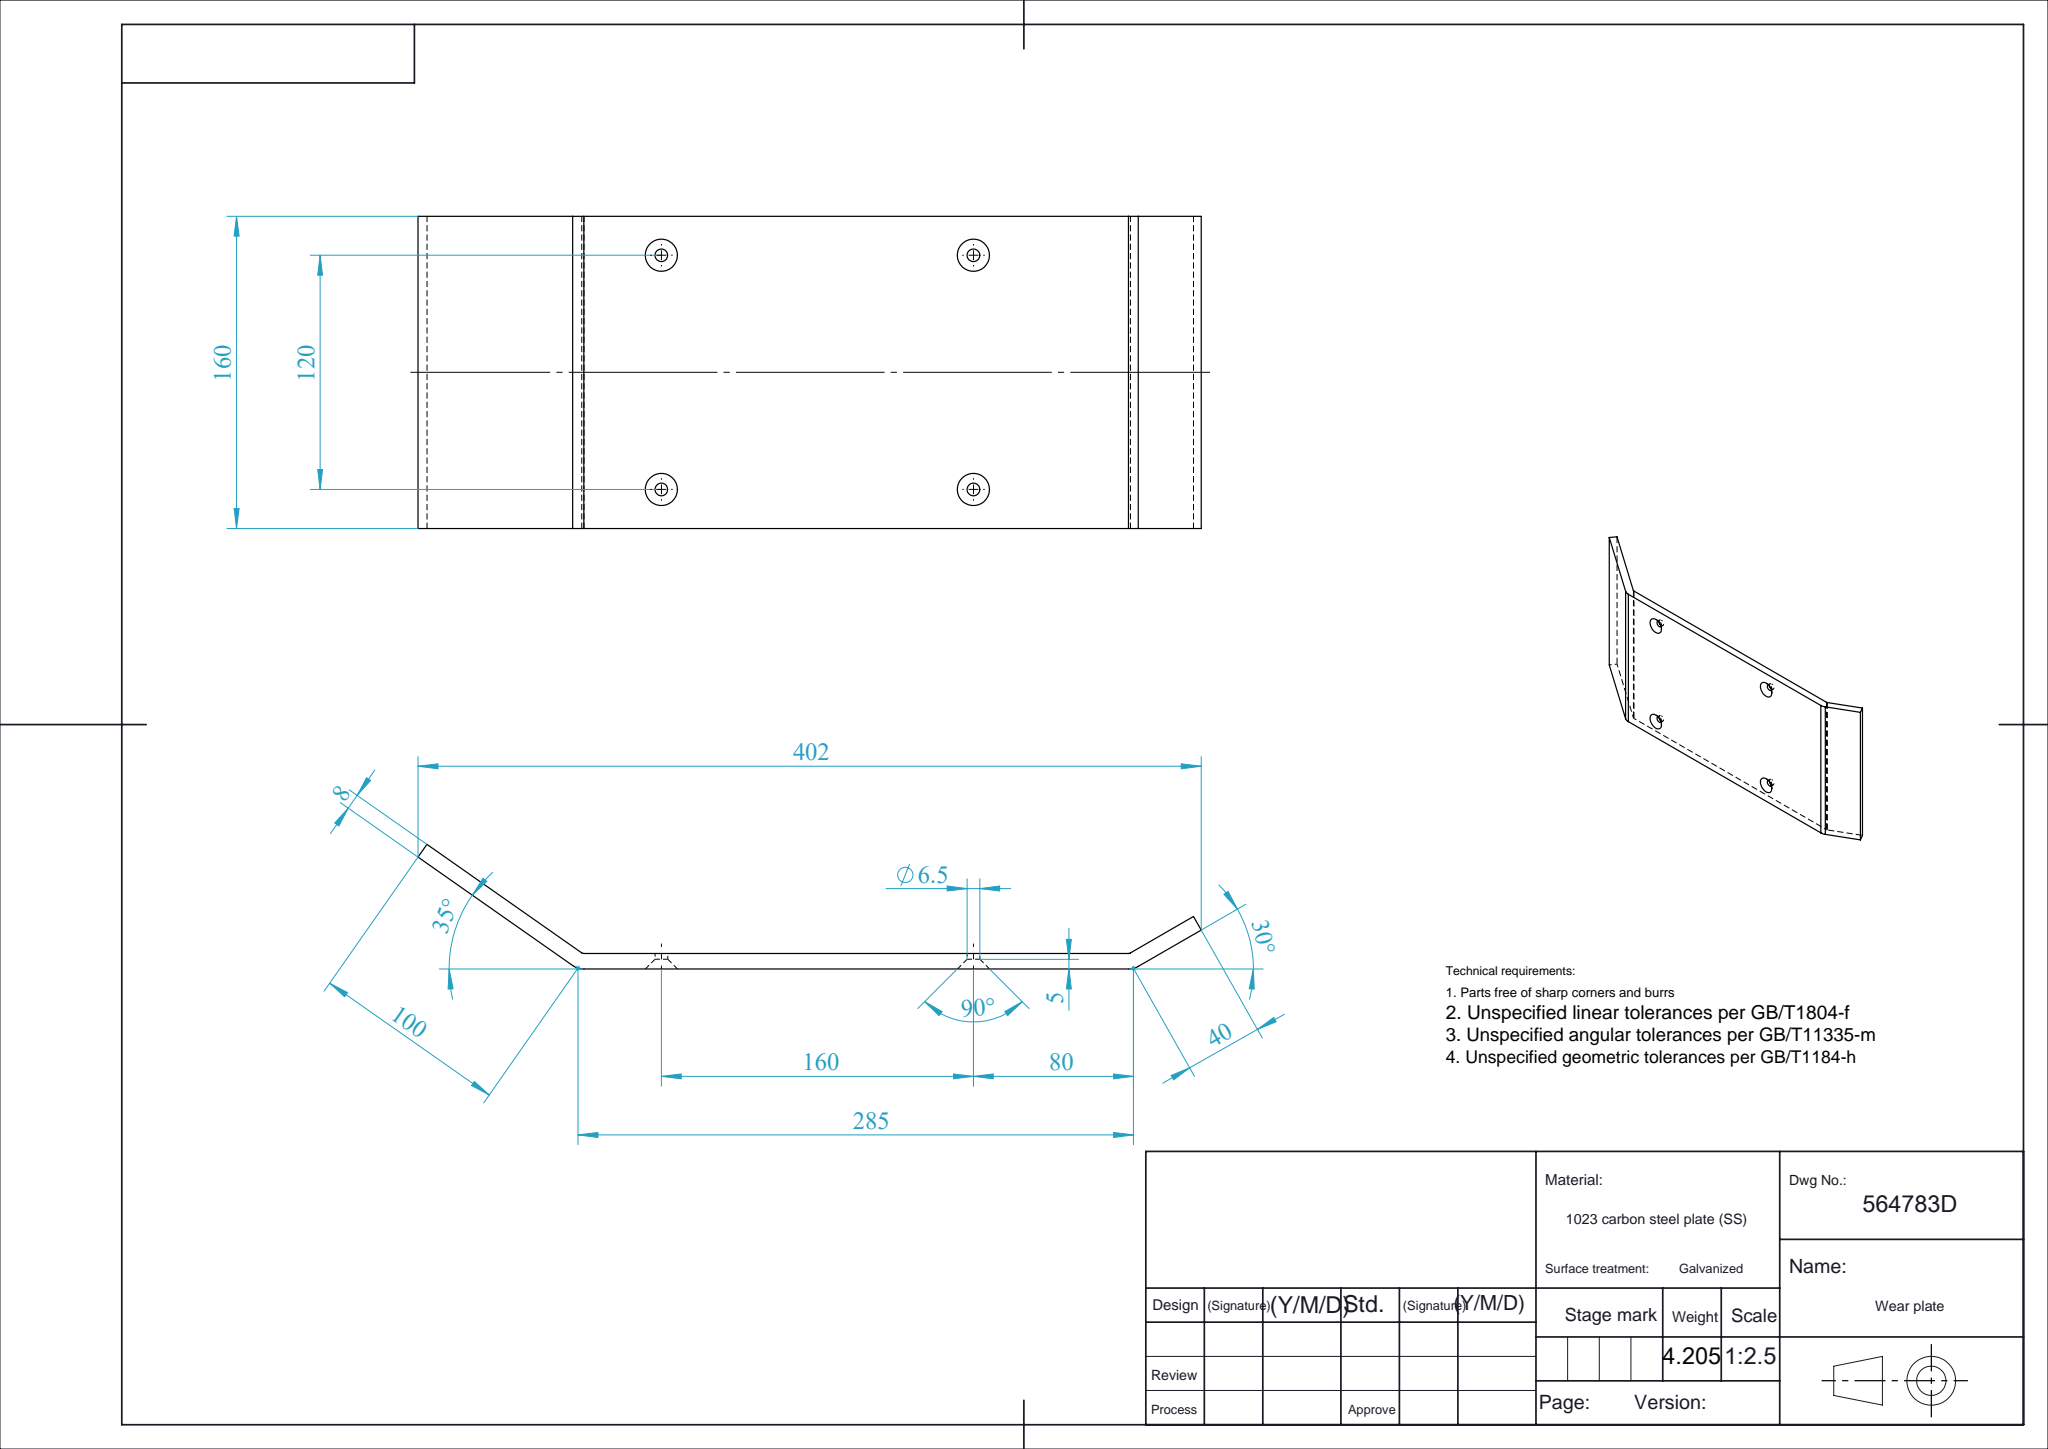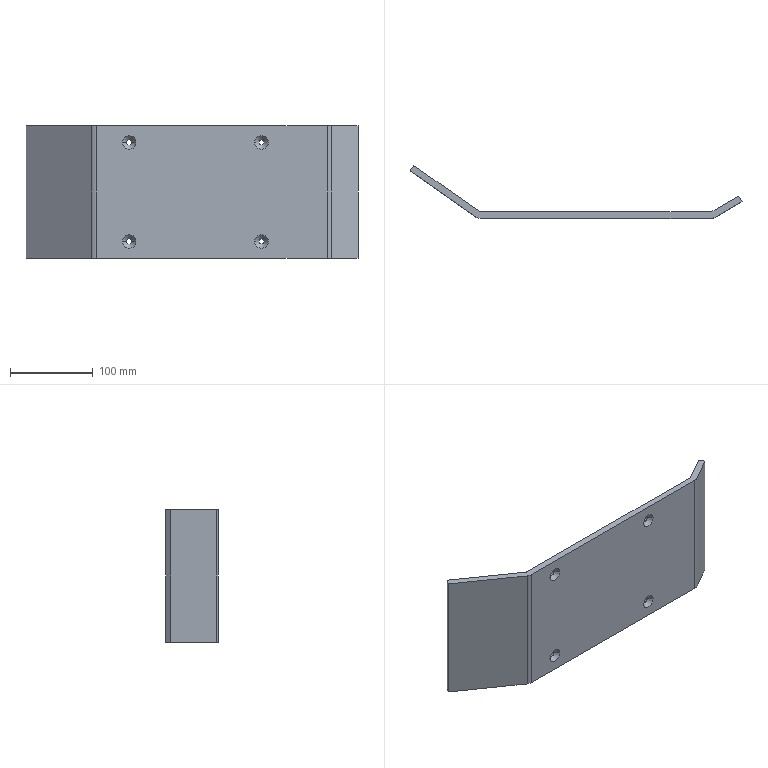Part | SolidWorks | features Fillet 2, ICE 2, Extrusion 1 | 1 solid | 30 faces | box 401.556 x 63.911 x 160 mm | volume 535175 mm3 | cylinder 12 | plane 10 | cone 8 | commonest cylinder face diameters 6.5 x8 4 x2 20 x2
STEP:
#1=CARTESIAN_POINT('',(121.522,-52.358,20.));
#2=VERTEX_POINT('',#1);
#3=CARTESIAN_POINT('',(124.772,-52.358,16.75));
#4=VERTEX_POINT('',#3);
#5=CARTESIAN_POINT('',(124.772,-52.358,20.));
#6=DIRECTION('',(0.,-1.,0.));
#7=DIRECTION('',(1.,0.,0.));
#8=AXIS2_PLACEMENT_3D('',#5,#6,#7);
#9=CIRCLE('',#8,3.25);
#10=EDGE_CURVE('',#2,#4,#9,.T.);
#11=ORIENTED_EDGE('',*,*,#10,.F.);
#12=CARTESIAN_POINT('',(116.522,-57.358,20.));
#13=VERTEX_POINT('',#12);
#14=CARTESIAN_POINT('',(116.522,-57.358,20.));
#15=DIRECTION('',(-0.7071,-0.7071,0.));
#16=VECTOR('',#15,1000.);
#17=LINE('',#14,#16);
#18=EDGE_CURVE('',#2,#13,#17,.T.);
#19=ORIENTED_EDGE('',*,*,#18,.T.);
#20=CARTESIAN_POINT('',(133.022,-57.358,20.));
#21=VERTEX_POINT('',#20);
#22=CARTESIAN_POINT('',(124.772,-57.358,20.));
#23=DIRECTION('',(0.,-1.,0.));
#24=DIRECTION('',(1.,0.,0.));
#25=AXIS2_PLACEMENT_3D('',#22,#23,#24);
#26=CIRCLE('',#25,8.25);
#27=EDGE_CURVE('',#13,#21,#26,.T.);
#28=ORIENTED_EDGE('',*,*,#27,.T.);
#29=CARTESIAN_POINT('',(128.022,-52.358,20.));
#30=VERTEX_POINT('',#29);
#31=CARTESIAN_POINT('',(133.022,-57.358,20.));
#32=DIRECTION('',(0.7071,-0.7071,0.));
#33=VECTOR('',#32,1000.);
#34=LINE('',#31,#33);
#35=EDGE_CURVE('',#30,#21,#34,.T.);
#36=ORIENTED_EDGE('',*,*,#35,.F.);
#37=CARTESIAN_POINT('',(124.772,-52.358,20.));
#38=DIRECTION('',(0.,-1.,0.));
#39=DIRECTION('',(1.,0.,0.));
#40=AXIS2_PLACEMENT_3D('',#37,#38,#39);
#41=CIRCLE('',#40,3.25);
#42=EDGE_CURVE('',#4,#30,#41,.T.);
#43=ORIENTED_EDGE('',*,*,#42,.F.);
#44=EDGE_LOOP('',(#11,#19,#28,#36,#43));
#45=FACE_OUTER_BOUND('',#44,.T.);
#46=CARTESIAN_POINT('',(124.772,-57.358,20.));
#47=DIRECTION('',(0.,-1.,0.));
#48=DIRECTION('',(1.,0.,0.));
#49=AXIS2_PLACEMENT_3D('',#46,#47,#48);
#50=CONICAL_SURFACE('',#49,8.25,0.7854);
#51=ADVANCED_FACE('',(#45),#50,.F.);
#52=CARTESIAN_POINT('',(281.522,-52.358,140.));
#53=VERTEX_POINT('',#52);
#54=CARTESIAN_POINT('',(284.772,-52.358,136.75));
#55=VERTEX_POINT('',#54);
#56=CARTESIAN_POINT('',(284.772,-52.358,140.));
#57=DIRECTION('',(0.,-1.,0.));
#58=DIRECTION('',(1.,0.,0.));
#59=AXIS2_PLACEMENT_3D('',#56,#57,#58);
#60=CIRCLE('',#59,3.25);
#61=EDGE_CURVE('',#53,#55,#60,.T.);
#62=ORIENTED_EDGE('',*,*,#61,.F.);
#63=CARTESIAN_POINT('',(276.522,-57.358,140.));
#64=VERTEX_POINT('',#63);
#65=CARTESIAN_POINT('',(276.522,-57.358,140.));
#66=DIRECTION('',(-0.7071,-0.7071,0.));
#67=VECTOR('',#66,1000.);
#68=LINE('',#65,#67);
#69=EDGE_CURVE('',#53,#64,#68,.T.);
#70=ORIENTED_EDGE('',*,*,#69,.T.);
#71=CARTESIAN_POINT('',(293.022,-57.358,140.));
#72=VERTEX_POINT('',#71);
#73=CARTESIAN_POINT('',(284.772,-57.358,140.));
#74=DIRECTION('',(0.,-1.,0.));
#75=DIRECTION('',(1.,0.,0.));
#76=AXIS2_PLACEMENT_3D('',#73,#74,#75);
#77=CIRCLE('',#76,8.25);
#78=EDGE_CURVE('',#64,#72,#77,.T.);
#79=ORIENTED_EDGE('',*,*,#78,.T.);
#80=CARTESIAN_POINT('',(288.022,-52.358,140.));
#81=VERTEX_POINT('',#80);
#82=CARTESIAN_POINT('',(293.022,-57.358,140.));
#83=DIRECTION('',(0.7071,-0.7071,0.));
#84=VECTOR('',#83,1000.);
#85=LINE('',#82,#84);
#86=EDGE_CURVE('',#81,#72,#85,.T.);
#87=ORIENTED_EDGE('',*,*,#86,.F.);
#88=CARTESIAN_POINT('',(284.772,-52.358,140.));
#89=DIRECTION('',(0.,-1.,0.));
#90=DIRECTION('',(1.,0.,0.));
#91=AXIS2_PLACEMENT_3D('',#88,#89,#90);
#92=CIRCLE('',#91,3.25);
#93=EDGE_CURVE('',#55,#81,#92,.T.);
#94=ORIENTED_EDGE('',*,*,#93,.F.);
#95=EDGE_LOOP('',(#62,#70,#79,#87,#94));
#96=FACE_OUTER_BOUND('',#95,.T.);
#97=CARTESIAN_POINT('',(284.772,-57.358,140.));
#98=DIRECTION('',(0.,-1.,0.));
#99=DIRECTION('',(1.,0.,0.));
#100=AXIS2_PLACEMENT_3D('',#97,#98,#99);
#101=CONICAL_SURFACE('',#100,8.25,0.7854);
#102=ADVANCED_FACE('',(#96),#101,.F.);
#103=CARTESIAN_POINT('',(121.522,-52.358,140.));
#104=VERTEX_POINT('',#103);
#105=CARTESIAN_POINT('',(124.772,-52.358,136.75));
#106=VERTEX_POINT('',#105);
#107=CARTESIAN_POINT('',(124.772,-52.358,140.));
#108=DIRECTION('',(0.,-1.,0.));
#109=DIRECTION('',(1.,0.,0.));
#110=AXIS2_PLACEMENT_3D('',#107,#108,#109);
#111=CIRCLE('',#110,3.25);
#112=EDGE_CURVE('',#104,#106,#111,.T.);
#113=ORIENTED_EDGE('',*,*,#112,.F.);
#114=CARTESIAN_POINT('',(116.522,-57.358,140.));
#115=VERTEX_POINT('',#114);
#116=CARTESIAN_POINT('',(116.522,-57.358,140.));
#117=DIRECTION('',(-0.7071,-0.7071,0.));
#118=VECTOR('',#117,1000.);
#119=LINE('',#116,#118);
#120=EDGE_CURVE('',#104,#115,#119,.T.);
#121=ORIENTED_EDGE('',*,*,#120,.T.);
#122=CARTESIAN_POINT('',(133.022,-57.358,140.));
#123=VERTEX_POINT('',#122);
#124=CARTESIAN_POINT('',(124.772,-57.358,140.));
#125=DIRECTION('',(0.,-1.,0.));
#126=DIRECTION('',(1.,0.,0.));
#127=AXIS2_PLACEMENT_3D('',#124,#125,#126);
#128=CIRCLE('',#127,8.25);
#129=EDGE_CURVE('',#115,#123,#128,.T.);
#130=ORIENTED_EDGE('',*,*,#129,.T.);
#131=CARTESIAN_POINT('',(128.022,-52.358,140.));
#132=VERTEX_POINT('',#131);
#133=CARTESIAN_POINT('',(133.022,-57.358,140.));
#134=DIRECTION('',(0.7071,-0.7071,0.));
#135=VECTOR('',#134,1000.);
#136=LINE('',#133,#135);
#137=EDGE_CURVE('',#132,#123,#136,.T.);
#138=ORIENTED_EDGE('',*,*,#137,.F.);
#139=CARTESIAN_POINT('',(124.772,-52.358,140.));
#140=DIRECTION('',(0.,-1.,0.));
#141=DIRECTION('',(1.,0.,0.));
#142=AXIS2_PLACEMENT_3D('',#139,#140,#141);
#143=CIRCLE('',#142,3.25);
#144=EDGE_CURVE('',#106,#132,#143,.T.);
#145=ORIENTED_EDGE('',*,*,#144,.F.);
#146=EDGE_LOOP('',(#113,#121,#130,#138,#145));
#147=FACE_OUTER_BOUND('',#146,.T.);
#148=CARTESIAN_POINT('',(124.772,-57.358,140.));
#149=DIRECTION('',(0.,-1.,0.));
#150=DIRECTION('',(1.,0.,0.));
#151=AXIS2_PLACEMENT_3D('',#148,#149,#150);
#152=CONICAL_SURFACE('',#151,8.25,0.7854);
#153=ADVANCED_FACE('',(#147),#152,.F.);
#154=CARTESIAN_POINT('',(281.522,-52.358,20.));
#155=VERTEX_POINT('',#154);
#156=CARTESIAN_POINT('',(284.772,-52.358,16.75));
#157=VERTEX_POINT('',#156);
#158=CARTESIAN_POINT('',(284.772,-52.358,20.));
#159=DIRECTION('',(0.,-1.,0.));
#160=DIRECTION('',(1.,0.,0.));
#161=AXIS2_PLACEMENT_3D('',#158,#159,#160);
#162=CIRCLE('',#161,3.25);
#163=EDGE_CURVE('',#155,#157,#162,.T.);
#164=ORIENTED_EDGE('',*,*,#163,.F.);
#165=CARTESIAN_POINT('',(276.522,-57.358,20.));
#166=VERTEX_POINT('',#165);
#167=CARTESIAN_POINT('',(276.522,-57.358,20.));
#168=DIRECTION('',(-0.7071,-0.7071,0.));
#169=VECTOR('',#168,1000.);
#170=LINE('',#167,#169);
#171=EDGE_CURVE('',#155,#166,#170,.T.);
#172=ORIENTED_EDGE('',*,*,#171,.T.);
#173=CARTESIAN_POINT('',(293.022,-57.358,20.));
#174=VERTEX_POINT('',#173);
#175=CARTESIAN_POINT('',(284.772,-57.358,20.));
#176=DIRECTION('',(0.,-1.,0.));
#177=DIRECTION('',(1.,0.,0.));
#178=AXIS2_PLACEMENT_3D('',#175,#176,#177);
#179=CIRCLE('',#178,8.25);
#180=EDGE_CURVE('',#166,#174,#179,.T.);
#181=ORIENTED_EDGE('',*,*,#180,.T.);
#182=CARTESIAN_POINT('',(288.022,-52.358,20.));
#183=VERTEX_POINT('',#182);
#184=CARTESIAN_POINT('',(293.022,-57.358,20.));
#185=DIRECTION('',(0.7071,-0.7071,0.));
#186=VECTOR('',#185,1000.);
#187=LINE('',#184,#186);
#188=EDGE_CURVE('',#183,#174,#187,.T.);
#189=ORIENTED_EDGE('',*,*,#188,.F.);
#190=CARTESIAN_POINT('',(284.772,-52.358,20.));
#191=DIRECTION('',(0.,-1.,0.));
#192=DIRECTION('',(1.,0.,0.));
#193=AXIS2_PLACEMENT_3D('',#190,#191,#192);
#194=CIRCLE('',#193,3.25);
#195=EDGE_CURVE('',#157,#183,#194,.T.);
#196=ORIENTED_EDGE('',*,*,#195,.F.);
#197=EDGE_LOOP('',(#164,#172,#181,#189,#196));
#198=FACE_OUTER_BOUND('',#197,.T.);
#199=CARTESIAN_POINT('',(284.772,-57.358,20.));
#200=DIRECTION('',(0.,-1.,0.));
#201=DIRECTION('',(1.,0.,0.));
#202=AXIS2_PLACEMENT_3D('',#199,#200,#201);
#203=CONICAL_SURFACE('',#202,8.25,0.7854);
#204=ADVANCED_FACE('',(#198),#203,.F.);
#205=CARTESIAN_POINT('',(284.772,-52.358,23.25));
#206=VERTEX_POINT('',#205);
#207=CARTESIAN_POINT('',(284.772,-52.358,20.));
#208=DIRECTION('',(0.,-1.,0.));
#209=DIRECTION('',(1.,0.,0.));
#210=AXIS2_PLACEMENT_3D('',#207,#208,#209);
#211=CIRCLE('',#210,3.25);
#212=EDGE_CURVE('',#206,#155,#211,.T.);
#213=ORIENTED_EDGE('',*,*,#212,.T.);
#214=ORIENTED_EDGE('',*,*,#163,.T.);
#215=CARTESIAN_POINT('',(284.772,-49.358,16.75));
#216=VERTEX_POINT('',#215);
#217=CARTESIAN_POINT('',(284.772,-57.358,16.75));
#218=DIRECTION('',(0.,1.,0.));
#219=VECTOR('',#218,1000.);
#220=LINE('',#217,#219);
#221=EDGE_CURVE('',#157,#216,#220,.T.);
#222=ORIENTED_EDGE('',*,*,#221,.T.);
#223=CARTESIAN_POINT('',(284.772,-49.358,23.25));
#224=VERTEX_POINT('',#223);
#225=CARTESIAN_POINT('',(284.772,-49.358,20.));
#226=DIRECTION('',(0.,1.,0.));
#227=DIRECTION('',(0.,0.,1.));
#228=AXIS2_PLACEMENT_3D('',#225,#226,#227);
#229=CIRCLE('',#228,3.25);
#230=EDGE_CURVE('',#216,#224,#229,.T.);
#231=ORIENTED_EDGE('',*,*,#230,.T.);
#232=CARTESIAN_POINT('',(284.772,-57.358,23.25));
#233=DIRECTION('',(0.,1.,0.));
#234=VECTOR('',#233,1000.);
#235=LINE('',#232,#234);
#236=EDGE_CURVE('',#206,#224,#235,.T.);
#237=ORIENTED_EDGE('',*,*,#236,.F.);
#238=EDGE_LOOP('',(#213,#214,#222,#231,#237));
#239=FACE_OUTER_BOUND('',#238,.T.);
#240=CARTESIAN_POINT('',(284.772,-57.358,20.));
#241=DIRECTION('',(0.,1.,0.));
#242=DIRECTION('',(0.,0.,1.));
#243=AXIS2_PLACEMENT_3D('',#240,#241,#242);
#244=CYLINDRICAL_SURFACE('',#243,3.25);
#245=ADVANCED_FACE('',(#239),#244,.F.);
#246=CARTESIAN_POINT('',(124.772,-52.358,143.25));
#247=VERTEX_POINT('',#246);
#248=CARTESIAN_POINT('',(124.772,-52.358,140.));
#249=DIRECTION('',(0.,-1.,0.));
#250=DIRECTION('',(1.,0.,0.));
#251=AXIS2_PLACEMENT_3D('',#248,#249,#250);
#252=CIRCLE('',#251,3.25);
#253=EDGE_CURVE('',#247,#104,#252,.T.);
#254=ORIENTED_EDGE('',*,*,#253,.T.);
#255=ORIENTED_EDGE('',*,*,#112,.T.);
#256=CARTESIAN_POINT('',(124.772,-49.358,136.75));
#257=VERTEX_POINT('',#256);
#258=CARTESIAN_POINT('',(124.772,-57.358,136.75));
#259=DIRECTION('',(0.,1.,0.));
#260=VECTOR('',#259,1000.);
#261=LINE('',#258,#260);
#262=EDGE_CURVE('',#106,#257,#261,.T.);
#263=ORIENTED_EDGE('',*,*,#262,.T.);
#264=CARTESIAN_POINT('',(124.772,-49.358,143.25));
#265=VERTEX_POINT('',#264);
#266=CARTESIAN_POINT('',(124.772,-49.358,140.));
#267=DIRECTION('',(0.,1.,0.));
#268=DIRECTION('',(0.,0.,1.));
#269=AXIS2_PLACEMENT_3D('',#266,#267,#268);
#270=CIRCLE('',#269,3.25);
#271=EDGE_CURVE('',#257,#265,#270,.T.);
#272=ORIENTED_EDGE('',*,*,#271,.T.);
#273=CARTESIAN_POINT('',(124.772,-57.358,143.25));
#274=DIRECTION('',(0.,1.,0.));
#275=VECTOR('',#274,1000.);
#276=LINE('',#273,#275);
#277=EDGE_CURVE('',#247,#265,#276,.T.);
#278=ORIENTED_EDGE('',*,*,#277,.F.);
#279=EDGE_LOOP('',(#254,#255,#263,#272,#278));
#280=FACE_OUTER_BOUND('',#279,.T.);
#281=CARTESIAN_POINT('',(124.772,-57.358,140.));
#282=DIRECTION('',(0.,1.,0.));
#283=DIRECTION('',(0.,0.,1.));
#284=AXIS2_PLACEMENT_3D('',#281,#282,#283);
#285=CYLINDRICAL_SURFACE('',#284,3.25);
#286=ADVANCED_FACE('',(#280),#285,.F.);
#287=CARTESIAN_POINT('',(284.772,-52.358,143.25));
#288=VERTEX_POINT('',#287);
#289=CARTESIAN_POINT('',(284.772,-52.358,140.));
#290=DIRECTION('',(0.,-1.,0.));
#291=DIRECTION('',(1.,0.,0.));
#292=AXIS2_PLACEMENT_3D('',#289,#290,#291);
#293=CIRCLE('',#292,3.25);
#294=EDGE_CURVE('',#288,#53,#293,.T.);
#295=ORIENTED_EDGE('',*,*,#294,.T.);
#296=ORIENTED_EDGE('',*,*,#61,.T.);
#297=CARTESIAN_POINT('',(284.772,-49.358,136.75));
#298=VERTEX_POINT('',#297);
#299=CARTESIAN_POINT('',(284.772,-57.358,136.75));
#300=DIRECTION('',(0.,1.,0.));
#301=VECTOR('',#300,1000.);
#302=LINE('',#299,#301);
#303=EDGE_CURVE('',#55,#298,#302,.T.);
#304=ORIENTED_EDGE('',*,*,#303,.T.);
#305=CARTESIAN_POINT('',(284.772,-49.358,143.25));
#306=VERTEX_POINT('',#305);
#307=CARTESIAN_POINT('',(284.772,-49.358,140.));
#308=DIRECTION('',(0.,1.,0.));
#309=DIRECTION('',(0.,0.,1.));
#310=AXIS2_PLACEMENT_3D('',#307,#308,#309);
#311=CIRCLE('',#310,3.25);
#312=EDGE_CURVE('',#298,#306,#311,.T.);
#313=ORIENTED_EDGE('',*,*,#312,.T.);
#314=CARTESIAN_POINT('',(284.772,-57.358,143.25));
#315=DIRECTION('',(0.,1.,0.));
#316=VECTOR('',#315,1000.);
#317=LINE('',#314,#316);
#318=EDGE_CURVE('',#288,#306,#317,.T.);
#319=ORIENTED_EDGE('',*,*,#318,.F.);
#320=EDGE_LOOP('',(#295,#296,#304,#313,#319));
#321=FACE_OUTER_BOUND('',#320,.T.);
#322=CARTESIAN_POINT('',(284.772,-57.358,140.));
#323=DIRECTION('',(0.,1.,0.));
#324=DIRECTION('',(0.,0.,1.));
#325=AXIS2_PLACEMENT_3D('',#322,#323,#324);
#326=CYLINDRICAL_SURFACE('',#325,3.25);
#327=ADVANCED_FACE('',(#321),#326,.F.);
#328=CARTESIAN_POINT('',(124.772,-52.358,23.25));
#329=VERTEX_POINT('',#328);
#330=CARTESIAN_POINT('',(124.772,-52.358,20.));
#331=DIRECTION('',(0.,-1.,0.));
#332=DIRECTION('',(1.,0.,0.));
#333=AXIS2_PLACEMENT_3D('',#330,#331,#332);
#334=CIRCLE('',#333,3.25);
#335=EDGE_CURVE('',#329,#2,#334,.T.);
#336=ORIENTED_EDGE('',*,*,#335,.T.);
#337=ORIENTED_EDGE('',*,*,#10,.T.);
#338=CARTESIAN_POINT('',(124.772,-49.358,16.75));
#339=VERTEX_POINT('',#338);
#340=CARTESIAN_POINT('',(124.772,-57.358,16.75));
#341=DIRECTION('',(0.,1.,0.));
#342=VECTOR('',#341,1000.);
#343=LINE('',#340,#342);
#344=EDGE_CURVE('',#4,#339,#343,.T.);
#345=ORIENTED_EDGE('',*,*,#344,.T.);
#346=CARTESIAN_POINT('',(124.772,-49.358,23.25));
#347=VERTEX_POINT('',#346);
#348=CARTESIAN_POINT('',(124.772,-49.358,20.));
#349=DIRECTION('',(0.,1.,0.));
#350=DIRECTION('',(0.,0.,1.));
#351=AXIS2_PLACEMENT_3D('',#348,#349,#350);
#352=CIRCLE('',#351,3.25);
#353=EDGE_CURVE('',#339,#347,#352,.T.);
#354=ORIENTED_EDGE('',*,*,#353,.T.);
#355=CARTESIAN_POINT('',(124.772,-57.358,23.25));
#356=DIRECTION('',(0.,1.,0.));
#357=VECTOR('',#356,1000.);
#358=LINE('',#355,#357);
#359=EDGE_CURVE('',#329,#347,#358,.T.);
#360=ORIENTED_EDGE('',*,*,#359,.F.);
#361=EDGE_LOOP('',(#336,#337,#345,#354,#360));
#362=FACE_OUTER_BOUND('',#361,.T.);
#363=CARTESIAN_POINT('',(124.772,-57.358,20.));
#364=DIRECTION('',(0.,1.,0.));
#365=DIRECTION('',(0.,0.,1.));
#366=AXIS2_PLACEMENT_3D('',#363,#364,#365);
#367=CYLINDRICAL_SURFACE('',#366,3.25);
#368=ADVANCED_FACE('',(#362),#367,.F.);
#369=ORIENTED_EDGE('',*,*,#344,.F.);
#370=ORIENTED_EDGE('',*,*,#42,.T.);
#371=CARTESIAN_POINT('',(124.772,-52.358,20.));
#372=DIRECTION('',(0.,-1.,0.));
#373=DIRECTION('',(1.,0.,0.));
#374=AXIS2_PLACEMENT_3D('',#371,#372,#373);
#375=CIRCLE('',#374,3.25);
#376=EDGE_CURVE('',#30,#329,#375,.T.);
#377=ORIENTED_EDGE('',*,*,#376,.T.);
#378=ORIENTED_EDGE('',*,*,#359,.T.);
#379=CARTESIAN_POINT('',(124.772,-49.358,20.));
#380=DIRECTION('',(0.,1.,0.));
#381=DIRECTION('',(0.,0.,1.));
#382=AXIS2_PLACEMENT_3D('',#379,#380,#381);
#383=CIRCLE('',#382,3.25);
#384=EDGE_CURVE('',#347,#339,#383,.T.);
#385=ORIENTED_EDGE('',*,*,#384,.T.);
#386=EDGE_LOOP('',(#369,#370,#377,#378,#385));
#387=FACE_OUTER_BOUND('',#386,.T.);
#388=CARTESIAN_POINT('',(124.772,-57.358,20.));
#389=DIRECTION('',(0.,1.,0.));
#390=DIRECTION('',(0.,0.,1.));
#391=AXIS2_PLACEMENT_3D('',#388,#389,#390);
#392=CYLINDRICAL_SURFACE('',#391,3.25);
#393=ADVANCED_FACE('',(#387),#392,.F.);
#394=ORIENTED_EDGE('',*,*,#303,.F.);
#395=ORIENTED_EDGE('',*,*,#93,.T.);
#396=CARTESIAN_POINT('',(284.772,-52.358,140.));
#397=DIRECTION('',(0.,-1.,0.));
#398=DIRECTION('',(1.,0.,0.));
#399=AXIS2_PLACEMENT_3D('',#396,#397,#398);
#400=CIRCLE('',#399,3.25);
#401=EDGE_CURVE('',#81,#288,#400,.T.);
#402=ORIENTED_EDGE('',*,*,#401,.T.);
#403=ORIENTED_EDGE('',*,*,#318,.T.);
#404=CARTESIAN_POINT('',(284.772,-49.358,140.));
#405=DIRECTION('',(0.,1.,0.));
#406=DIRECTION('',(0.,0.,1.));
#407=AXIS2_PLACEMENT_3D('',#404,#405,#406);
#408=CIRCLE('',#407,3.25);
#409=EDGE_CURVE('',#306,#298,#408,.T.);
#410=ORIENTED_EDGE('',*,*,#409,.T.);
#411=EDGE_LOOP('',(#394,#395,#402,#403,#410));
#412=FACE_OUTER_BOUND('',#411,.T.);
#413=CARTESIAN_POINT('',(284.772,-57.358,140.));
#414=DIRECTION('',(0.,1.,0.));
#415=DIRECTION('',(0.,0.,1.));
#416=AXIS2_PLACEMENT_3D('',#413,#414,#415);
#417=CYLINDRICAL_SURFACE('',#416,3.25);
#418=ADVANCED_FACE('',(#412),#417,.F.);
#419=ORIENTED_EDGE('',*,*,#262,.F.);
#420=ORIENTED_EDGE('',*,*,#144,.T.);
#421=CARTESIAN_POINT('',(124.772,-52.358,140.));
#422=DIRECTION('',(0.,-1.,0.));
#423=DIRECTION('',(1.,0.,0.));
#424=AXIS2_PLACEMENT_3D('',#421,#422,#423);
#425=CIRCLE('',#424,3.25);
#426=EDGE_CURVE('',#132,#247,#425,.T.);
#427=ORIENTED_EDGE('',*,*,#426,.T.);
#428=ORIENTED_EDGE('',*,*,#277,.T.);
#429=CARTESIAN_POINT('',(124.772,-49.358,140.));
#430=DIRECTION('',(0.,1.,0.));
#431=DIRECTION('',(0.,0.,1.));
#432=AXIS2_PLACEMENT_3D('',#429,#430,#431);
#433=CIRCLE('',#432,3.25);
#434=EDGE_CURVE('',#265,#257,#433,.T.);
#435=ORIENTED_EDGE('',*,*,#434,.T.);
#436=EDGE_LOOP('',(#419,#420,#427,#428,#435));
#437=FACE_OUTER_BOUND('',#436,.T.);
#438=CARTESIAN_POINT('',(124.772,-57.358,140.));
#439=DIRECTION('',(0.,1.,0.));
#440=DIRECTION('',(0.,0.,1.));
#441=AXIS2_PLACEMENT_3D('',#438,#439,#440);
#442=CYLINDRICAL_SURFACE('',#441,3.25);
#443=ADVANCED_FACE('',(#437),#442,.F.);
#444=ORIENTED_EDGE('',*,*,#221,.F.);
#445=ORIENTED_EDGE('',*,*,#195,.T.);
#446=CARTESIAN_POINT('',(284.772,-52.358,20.));
#447=DIRECTION('',(0.,-1.,0.));
#448=DIRECTION('',(1.,0.,0.));
#449=AXIS2_PLACEMENT_3D('',#446,#447,#448);
#450=CIRCLE('',#449,3.25);
#451=EDGE_CURVE('',#183,#206,#450,.T.);
#452=ORIENTED_EDGE('',*,*,#451,.T.);
#453=ORIENTED_EDGE('',*,*,#236,.T.);
#454=CARTESIAN_POINT('',(284.772,-49.358,20.));
#455=DIRECTION('',(0.,1.,0.));
#456=DIRECTION('',(0.,0.,1.));
#457=AXIS2_PLACEMENT_3D('',#454,#455,#456);
#458=CIRCLE('',#457,3.25);
#459=EDGE_CURVE('',#224,#216,#458,.T.);
#460=ORIENTED_EDGE('',*,*,#459,.T.);
#461=EDGE_LOOP('',(#444,#445,#452,#453,#460));
#462=FACE_OUTER_BOUND('',#461,.T.);
#463=CARTESIAN_POINT('',(284.772,-57.358,20.));
#464=DIRECTION('',(0.,1.,0.));
#465=DIRECTION('',(0.,0.,1.));
#466=AXIS2_PLACEMENT_3D('',#463,#464,#465);
#467=CYLINDRICAL_SURFACE('',#466,3.25);
#468=ADVANCED_FACE('',(#462),#467,.F.);
#469=CARTESIAN_POINT('',(397.556,-30.429,0.));
#470=VERTEX_POINT('',#469);
#471=CARTESIAN_POINT('',(401.556,-37.358,0.));
#472=VERTEX_POINT('',#471);
#473=CARTESIAN_POINT('',(284.991,164.54,0.));
#474=DIRECTION('',(0.5,-0.866,0.));
#475=VECTOR('',#474,1000.);
#476=LINE('',#473,#475);
#477=EDGE_CURVE('',#470,#472,#476,.T.);
#478=ORIENTED_EDGE('',*,*,#477,.F.);
#479=CARTESIAN_POINT('',(397.556,-30.429,160.));
#480=VERTEX_POINT('',#479);
#481=CARTESIAN_POINT('',(397.556,-30.429,160.));
#482=DIRECTION('',(0.,0.,-1.));
#483=VECTOR('',#482,1000.);
#484=LINE('',#481,#483);
#485=EDGE_CURVE('',#480,#470,#484,.T.);
#486=ORIENTED_EDGE('',*,*,#485,.F.);
#487=CARTESIAN_POINT('',(401.556,-37.358,160.));
#488=VERTEX_POINT('',#487);
#489=CARTESIAN_POINT('',(284.991,164.54,160.));
#490=DIRECTION('',(0.5,-0.866,0.));
#491=VECTOR('',#490,1000.);
#492=LINE('',#489,#491);
#493=EDGE_CURVE('',#480,#488,#492,.T.);
#494=ORIENTED_EDGE('',*,*,#493,.T.);
#495=CARTESIAN_POINT('',(401.556,-37.358,160.));
#496=DIRECTION('',(0.,0.,-1.));
#497=VECTOR('',#496,1000.);
#498=LINE('',#495,#497);
#499=EDGE_CURVE('',#488,#472,#498,.T.);
#500=ORIENTED_EDGE('',*,*,#499,.T.);
#501=EDGE_LOOP('',(#478,#486,#494,#500));
#502=FACE_OUTER_BOUND('',#501,.T.);
#503=CARTESIAN_POINT('',(284.991,164.54,160.));
#504=DIRECTION('',(0.866,0.5,0.));
#505=DIRECTION('',(-0.5,0.866,0.));
#506=AXIS2_PLACEMENT_3D('',#503,#504,#505);
#507=PLANE('',#506);
#508=ADVANCED_FACE('',(#502),#507,.T.);
#509=CARTESIAN_POINT('',(365.236,-49.09,0.));
#510=VERTEX_POINT('',#509);
#511=CARTESIAN_POINT('',(112.565,-194.969,0.));
#512=DIRECTION('',(0.866,0.5,0.));
#513=VECTOR('',#512,1000.);
#514=LINE('',#511,#513);
#515=EDGE_CURVE('',#510,#470,#514,.T.);
#516=ORIENTED_EDGE('',*,*,#515,.F.);
#517=CARTESIAN_POINT('',(365.236,-49.09,160.));
#518=VERTEX_POINT('',#517);
#519=CARTESIAN_POINT('',(365.236,-49.09,160.));
#520=DIRECTION('',(0.,0.,1.));
#521=VECTOR('',#520,1000.);
#522=LINE('',#519,#521);
#523=EDGE_CURVE('',#510,#518,#522,.T.);
#524=ORIENTED_EDGE('',*,*,#523,.T.);
#525=CARTESIAN_POINT('',(112.565,-194.969,160.));
#526=DIRECTION('',(0.866,0.5,0.));
#527=VECTOR('',#526,1000.);
#528=LINE('',#525,#527);
#529=EDGE_CURVE('',#518,#480,#528,.T.);
#530=ORIENTED_EDGE('',*,*,#529,.T.);
#531=ORIENTED_EDGE('',*,*,#485,.T.);
#532=EDGE_LOOP('',(#516,#524,#530,#531));
#533=FACE_OUTER_BOUND('',#532,.T.);
#534=CARTESIAN_POINT('',(112.565,-194.969,160.));
#535=DIRECTION('',(-0.5,0.866,0.));
#536=DIRECTION('',(-0.866,-0.5,0.));
#537=AXIS2_PLACEMENT_3D('',#534,#535,#536);
#538=PLANE('',#537);
#539=ADVANCED_FACE('',(#533),#538,.T.);
#540=ORIENTED_EDGE('',*,*,#459,.F.);
#541=ORIENTED_EDGE('',*,*,#230,.F.);
#542=EDGE_LOOP('',(#540,#541));
#543=FACE_BOUND('',#542,.T.);
#544=ORIENTED_EDGE('',*,*,#434,.F.);
#545=ORIENTED_EDGE('',*,*,#271,.F.);
#546=EDGE_LOOP('',(#544,#545));
#547=FACE_BOUND('',#546,.T.);
#548=ORIENTED_EDGE('',*,*,#409,.F.);
#549=ORIENTED_EDGE('',*,*,#312,.F.);
#550=EDGE_LOOP('',(#548,#549));
#551=FACE_BOUND('',#550,.T.);
#552=ORIENTED_EDGE('',*,*,#384,.F.);
#553=ORIENTED_EDGE('',*,*,#353,.F.);
#554=EDGE_LOOP('',(#552,#553));
#555=FACE_BOUND('',#554,.T.);
#556=CARTESIAN_POINT('',(85.068,-49.358,0.));
#557=VERTEX_POINT('',#556);
#558=CARTESIAN_POINT('',(364.236,-49.358,0.));
#559=VERTEX_POINT('',#558);
#560=CARTESIAN_POINT('',(0.,-49.358,0.));
#561=DIRECTION('',(1.,0.,0.));
#562=VECTOR('',#561,1000.);
#563=LINE('',#560,#562);
#564=EDGE_CURVE('',#557,#559,#563,.T.);
#565=ORIENTED_EDGE('',*,*,#564,.F.);
#566=CARTESIAN_POINT('',(85.068,-49.358,160.));
#567=VERTEX_POINT('',#566);
#568=CARTESIAN_POINT('',(85.068,-49.358,160.));
#569=DIRECTION('',(0.,0.,1.));
#570=VECTOR('',#569,1000.);
#571=LINE('',#568,#570);
#572=EDGE_CURVE('',#557,#567,#571,.T.);
#573=ORIENTED_EDGE('',*,*,#572,.T.);
#574=CARTESIAN_POINT('',(364.236,-49.358,160.));
#575=VERTEX_POINT('',#574);
#576=CARTESIAN_POINT('',(0.,-49.358,160.));
#577=DIRECTION('',(1.,0.,0.));
#578=VECTOR('',#577,1000.);
#579=LINE('',#576,#578);
#580=EDGE_CURVE('',#567,#575,#579,.T.);
#581=ORIENTED_EDGE('',*,*,#580,.T.);
#582=CARTESIAN_POINT('',(364.236,-49.358,0.));
#583=DIRECTION('',(0.,0.,-1.));
#584=VECTOR('',#583,1000.);
#585=LINE('',#582,#584);
#586=EDGE_CURVE('',#575,#559,#585,.T.);
#587=ORIENTED_EDGE('',*,*,#586,.T.);
#588=EDGE_LOOP('',(#565,#573,#581,#587));
#589=FACE_OUTER_BOUND('',#588,.T.);
#590=CARTESIAN_POINT('',(0.,-49.358,160.));
#591=DIRECTION('',(0.,1.,0.));
#592=DIRECTION('',(0.,0.,1.));
#593=AXIS2_PLACEMENT_3D('',#590,#591,#592);
#594=PLANE('',#593);
#595=ADVANCED_FACE('',(#543,#547,#551,#555,#589),#594,.T.);
#596=CARTESIAN_POINT('',(4.589,6.553,160.));
#597=VERTEX_POINT('',#596);
#598=CARTESIAN_POINT('',(83.921,-48.996,160.));
#599=VERTEX_POINT('',#598);
#600=CARTESIAN_POINT('',(4.589,6.553,160.));
#601=DIRECTION('',(0.8192,-0.5736,0.));
#602=VECTOR('',#601,1000.);
#603=LINE('',#600,#602);
#604=EDGE_CURVE('',#597,#599,#603,.T.);
#605=ORIENTED_EDGE('',*,*,#604,.T.);
#606=CARTESIAN_POINT('',(83.921,-48.996,0.));
#607=VERTEX_POINT('',#606);
#608=CARTESIAN_POINT('',(83.921,-48.996,0.));
#609=DIRECTION('',(0.,0.,-1.));
#610=VECTOR('',#609,1000.);
#611=LINE('',#608,#610);
#612=EDGE_CURVE('',#599,#607,#611,.T.);
#613=ORIENTED_EDGE('',*,*,#612,.T.);
#614=CARTESIAN_POINT('',(4.589,6.553,0.));
#615=VERTEX_POINT('',#614);
#616=CARTESIAN_POINT('',(4.589,6.553,0.));
#617=DIRECTION('',(0.8192,-0.5736,0.));
#618=VECTOR('',#617,1000.);
#619=LINE('',#616,#618);
#620=EDGE_CURVE('',#615,#607,#619,.T.);
#621=ORIENTED_EDGE('',*,*,#620,.F.);
#622=CARTESIAN_POINT('',(4.589,6.553,160.));
#623=DIRECTION('',(0.,0.,-1.));
#624=VECTOR('',#623,1000.);
#625=LINE('',#622,#624);
#626=EDGE_CURVE('',#597,#615,#625,.T.);
#627=ORIENTED_EDGE('',*,*,#626,.F.);
#628=EDGE_LOOP('',(#605,#613,#621,#627));
#629=FACE_OUTER_BOUND('',#628,.T.);
#630=CARTESIAN_POINT('',(4.589,6.553,160.));
#631=DIRECTION('',(0.5736,0.8192,0.));
#632=DIRECTION('',(-0.8192,0.5736,0.));
#633=AXIS2_PLACEMENT_3D('',#630,#631,#632);
#634=PLANE('',#633);
#635=ADVANCED_FACE('',(#629),#634,.T.);
#636=CARTESIAN_POINT('',(0.,0.,0.));
#637=VERTEX_POINT('',#636);
#638=CARTESIAN_POINT('',(0.,0.,0.));
#639=DIRECTION('',(-0.5736,-0.8192,0.));
#640=VECTOR('',#639,1000.);
#641=LINE('',#638,#640);
#642=EDGE_CURVE('',#615,#637,#641,.T.);
#643=ORIENTED_EDGE('',*,*,#642,.T.);
#644=CARTESIAN_POINT('',(0.,0.,160.));
#645=VERTEX_POINT('',#644);
#646=CARTESIAN_POINT('',(0.,0.,160.));
#647=DIRECTION('',(0.,0.,-1.));
#648=VECTOR('',#647,1000.);
#649=LINE('',#646,#648);
#650=EDGE_CURVE('',#645,#637,#649,.T.);
#651=ORIENTED_EDGE('',*,*,#650,.F.);
#652=CARTESIAN_POINT('',(0.,0.,160.));
#653=DIRECTION('',(-0.5736,-0.8192,0.));
#654=VECTOR('',#653,1000.);
#655=LINE('',#652,#654);
#656=EDGE_CURVE('',#597,#645,#655,.T.);
#657=ORIENTED_EDGE('',*,*,#656,.F.);
#658=ORIENTED_EDGE('',*,*,#626,.T.);
#659=EDGE_LOOP('',(#643,#651,#657,#658));
#660=FACE_OUTER_BOUND('',#659,.T.);
#661=CARTESIAN_POINT('',(0.,0.,160.));
#662=DIRECTION('',(0.8192,-0.5736,0.));
#663=DIRECTION('',(0.5736,0.8192,0.));
#664=AXIS2_PLACEMENT_3D('',#661,#662,#663);
#665=PLANE('',#664);
#666=ADVANCED_FACE('',(#660),#665,.F.);
#667=CARTESIAN_POINT('',(79.332,-55.549,0.));
#668=VERTEX_POINT('',#667);
#669=CARTESIAN_POINT('',(0.,0.,0.));
#670=DIRECTION('',(0.8192,-0.5736,0.));
#671=VECTOR('',#670,1000.);
#672=LINE('',#669,#671);
#673=EDGE_CURVE('',#637,#668,#672,.T.);
#674=ORIENTED_EDGE('',*,*,#673,.T.);
#675=CARTESIAN_POINT('',(79.332,-55.549,160.));
#676=VERTEX_POINT('',#675);
#677=CARTESIAN_POINT('',(79.332,-55.549,160.));
#678=DIRECTION('',(0.,0.,1.));
#679=VECTOR('',#678,1000.);
#680=LINE('',#677,#679);
#681=EDGE_CURVE('',#668,#676,#680,.T.);
#682=ORIENTED_EDGE('',*,*,#681,.T.);
#683=CARTESIAN_POINT('',(0.,0.,160.));
#684=DIRECTION('',(0.8192,-0.5736,0.));
#685=VECTOR('',#684,1000.);
#686=LINE('',#683,#685);
#687=EDGE_CURVE('',#645,#676,#686,.T.);
#688=ORIENTED_EDGE('',*,*,#687,.F.);
#689=ORIENTED_EDGE('',*,*,#650,.T.);
#690=EDGE_LOOP('',(#674,#682,#688,#689));
#691=FACE_OUTER_BOUND('',#690,.T.);
#692=CARTESIAN_POINT('',(0.,0.,160.));
#693=DIRECTION('',(0.5736,0.8192,0.));
#694=DIRECTION('',(-0.8192,0.5736,0.));
#695=AXIS2_PLACEMENT_3D('',#692,#693,#694);
#696=PLANE('',#695);
#697=ADVANCED_FACE('',(#691),#696,.F.);
#698=CARTESIAN_POINT('',(124.772,-57.358,20.));
#699=DIRECTION('',(0.,-1.,0.));
#700=DIRECTION('',(1.,0.,0.));
#701=AXIS2_PLACEMENT_3D('',#698,#699,#700);
#702=CIRCLE('',#701,8.25);
#703=EDGE_CURVE('',#21,#13,#702,.T.);
#704=ORIENTED_EDGE('',*,*,#703,.F.);
#705=ORIENTED_EDGE('',*,*,#27,.F.);
#706=EDGE_LOOP('',(#704,#705));
#707=FACE_BOUND('',#706,.T.);
#708=CARTESIAN_POINT('',(284.772,-57.358,20.));
#709=DIRECTION('',(0.,-1.,0.));
#710=DIRECTION('',(1.,0.,0.));
#711=AXIS2_PLACEMENT_3D('',#708,#709,#710);
#712=CIRCLE('',#711,8.25);
#713=EDGE_CURVE('',#174,#166,#712,.T.);
#714=ORIENTED_EDGE('',*,*,#713,.F.);
#715=ORIENTED_EDGE('',*,*,#180,.F.);
#716=EDGE_LOOP('',(#714,#715));
#717=FACE_BOUND('',#716,.T.);
#718=CARTESIAN_POINT('',(284.772,-57.358,140.));
#719=DIRECTION('',(0.,-1.,0.));
#720=DIRECTION('',(1.,0.,0.));
#721=AXIS2_PLACEMENT_3D('',#718,#719,#720);
#722=CIRCLE('',#721,8.25);
#723=EDGE_CURVE('',#72,#64,#722,.T.);
#724=ORIENTED_EDGE('',*,*,#723,.F.);
#725=ORIENTED_EDGE('',*,*,#78,.F.);
#726=EDGE_LOOP('',(#724,#725));
#727=FACE_BOUND('',#726,.T.);
#728=CARTESIAN_POINT('',(124.772,-57.358,140.));
#729=DIRECTION('',(0.,-1.,0.));
#730=DIRECTION('',(1.,0.,0.));
#731=AXIS2_PLACEMENT_3D('',#728,#729,#730);
#732=CIRCLE('',#731,8.25);
#733=EDGE_CURVE('',#123,#115,#732,.T.);
#734=ORIENTED_EDGE('',*,*,#733,.F.);
#735=ORIENTED_EDGE('',*,*,#129,.F.);
#736=EDGE_LOOP('',(#734,#735));
#737=FACE_BOUND('',#736,.T.);
#738=CARTESIAN_POINT('',(85.068,-57.358,0.));
#739=VERTEX_POINT('',#738);
#740=CARTESIAN_POINT('',(364.236,-57.358,0.));
#741=VERTEX_POINT('',#740);
#742=CARTESIAN_POINT('',(0.,-57.358,0.));
#743=DIRECTION('',(1.,0.,0.));
#744=VECTOR('',#743,1000.);
#745=LINE('',#742,#744);
#746=EDGE_CURVE('',#739,#741,#745,.T.);
#747=ORIENTED_EDGE('',*,*,#746,.T.);
#748=CARTESIAN_POINT('',(364.236,-57.358,160.));
#749=VERTEX_POINT('',#748);
#750=CARTESIAN_POINT('',(364.236,-57.358,160.));
#751=DIRECTION('',(0.,0.,1.));
#752=VECTOR('',#751,1000.);
#753=LINE('',#750,#752);
#754=EDGE_CURVE('',#741,#749,#753,.T.);
#755=ORIENTED_EDGE('',*,*,#754,.T.);
#756=CARTESIAN_POINT('',(85.068,-57.358,160.));
#757=VERTEX_POINT('',#756);
#758=CARTESIAN_POINT('',(0.,-57.358,160.));
#759=DIRECTION('',(1.,0.,0.));
#760=VECTOR('',#759,1000.);
#761=LINE('',#758,#760);
#762=EDGE_CURVE('',#757,#749,#761,.T.);
#763=ORIENTED_EDGE('',*,*,#762,.F.);
#764=CARTESIAN_POINT('',(85.068,-57.358,160.));
#765=DIRECTION('',(0.,0.,-1.));
#766=VECTOR('',#765,1000.);
#767=LINE('',#764,#766);
#768=EDGE_CURVE('',#757,#739,#767,.T.);
#769=ORIENTED_EDGE('',*,*,#768,.T.);
#770=EDGE_LOOP('',(#747,#755,#763,#769));
#771=FACE_OUTER_BOUND('',#770,.T.);
#772=CARTESIAN_POINT('',(0.,-57.358,160.));
#773=DIRECTION('',(0.,1.,0.));
#774=DIRECTION('',(-1.,0.,0.));
#775=AXIS2_PLACEMENT_3D('',#772,#773,#774);
#776=PLANE('',#775);
#777=ADVANCED_FACE('',(#707,#717,#727,#737,#771),#776,.F.);
#778=CARTESIAN_POINT('',(369.236,-56.018,160.));
#779=VERTEX_POINT('',#778);
#780=CARTESIAN_POINT('',(116.565,-201.897,160.));
#781=DIRECTION('',(0.866,0.5,0.));
#782=VECTOR('',#781,1000.);
#783=LINE('',#780,#782);
#784=EDGE_CURVE('',#779,#488,#783,.T.);
#785=ORIENTED_EDGE('',*,*,#784,.F.);
#786=CARTESIAN_POINT('',(369.236,-56.018,0.));
#787=VERTEX_POINT('',#786);
#788=CARTESIAN_POINT('',(369.236,-56.018,160.));
#789=DIRECTION('',(0.,0.,-1.));
#790=VECTOR('',#789,1000.);
#791=LINE('',#788,#790);
#792=EDGE_CURVE('',#779,#787,#791,.T.);
#793=ORIENTED_EDGE('',*,*,#792,.T.);
#794=CARTESIAN_POINT('',(116.565,-201.897,0.));
#795=DIRECTION('',(0.866,0.5,0.));
#796=VECTOR('',#795,1000.);
#797=LINE('',#794,#796);
#798=EDGE_CURVE('',#787,#472,#797,.T.);
#799=ORIENTED_EDGE('',*,*,#798,.T.);
#800=ORIENTED_EDGE('',*,*,#499,.F.);
#801=EDGE_LOOP('',(#785,#793,#799,#800));
#802=FACE_OUTER_BOUND('',#801,.T.);
#803=CARTESIAN_POINT('',(116.565,-201.897,160.));
#804=DIRECTION('',(-0.5,0.866,0.));
#805=DIRECTION('',(-0.866,-0.5,0.));
#806=AXIS2_PLACEMENT_3D('',#803,#804,#805);
#807=PLANE('',#806);
#808=ADVANCED_FACE('',(#802),#807,.F.);
#809=ORIENTED_EDGE('',*,*,#762,.T.);
#810=CARTESIAN_POINT('',(364.236,-47.358,160.));
#811=DIRECTION('',(0.,0.,1.));
#812=DIRECTION('',(1.,0.,0.));
#813=AXIS2_PLACEMENT_3D('',#810,#811,#812);
#814=CIRCLE('',#813,10.);
#815=EDGE_CURVE('',#749,#779,#814,.T.);
#816=ORIENTED_EDGE('',*,*,#815,.T.);
#817=ORIENTED_EDGE('',*,*,#784,.T.);
#818=ORIENTED_EDGE('',*,*,#493,.F.);
#819=ORIENTED_EDGE('',*,*,#529,.F.);
#820=CARTESIAN_POINT('',(364.236,-47.358,160.));
#821=DIRECTION('',(0.,0.,-1.));
#822=DIRECTION('',(1.,0.,0.));
#823=AXIS2_PLACEMENT_3D('',#820,#821,#822);
#824=CIRCLE('',#823,2.);
#825=EDGE_CURVE('',#518,#575,#824,.T.);
#826=ORIENTED_EDGE('',*,*,#825,.T.);
#827=ORIENTED_EDGE('',*,*,#580,.F.);
#828=CARTESIAN_POINT('',(85.068,-47.358,160.));
#829=DIRECTION('',(0.,0.,-1.));
#830=DIRECTION('',(1.,0.,0.));
#831=AXIS2_PLACEMENT_3D('',#828,#829,#830);
#832=CIRCLE('',#831,2.);
#833=EDGE_CURVE('',#567,#599,#832,.T.);
#834=ORIENTED_EDGE('',*,*,#833,.T.);
#835=ORIENTED_EDGE('',*,*,#604,.F.);
#836=ORIENTED_EDGE('',*,*,#656,.T.);
#837=ORIENTED_EDGE('',*,*,#687,.T.);
#838=CARTESIAN_POINT('',(85.068,-47.358,160.));
#839=DIRECTION('',(0.,0.,1.));
#840=DIRECTION('',(1.,0.,0.));
#841=AXIS2_PLACEMENT_3D('',#838,#839,#840);
#842=CIRCLE('',#841,10.);
#843=EDGE_CURVE('',#676,#757,#842,.T.);
#844=ORIENTED_EDGE('',*,*,#843,.T.);
#845=EDGE_LOOP('',(#809,#816,#817,#818,#819,#826,#827,#834,#835,#836,#837,#844));
#846=FACE_OUTER_BOUND('',#845,.T.);
#847=CARTESIAN_POINT('',(0.,0.,160.));
#848=DIRECTION('',(0.,0.,1.));
#849=DIRECTION('',(1.,0.,0.));
#850=AXIS2_PLACEMENT_3D('',#847,#848,#849);
#851=PLANE('',#850);
#852=ADVANCED_FACE('',(#846),#851,.T.);
#853=ORIENTED_EDGE('',*,*,#798,.F.);
#854=CARTESIAN_POINT('',(364.236,-47.358,0.));
#855=DIRECTION('',(0.,0.,-1.));
#856=DIRECTION('',(1.,0.,0.));
#857=AXIS2_PLACEMENT_3D('',#854,#855,#856);
#858=CIRCLE('',#857,10.);
#859=EDGE_CURVE('',#787,#741,#858,.T.);
#860=ORIENTED_EDGE('',*,*,#859,.T.);
#861=ORIENTED_EDGE('',*,*,#746,.F.);
#862=CARTESIAN_POINT('',(85.068,-47.358,0.));
#863=DIRECTION('',(0.,0.,-1.));
#864=DIRECTION('',(1.,0.,0.));
#865=AXIS2_PLACEMENT_3D('',#862,#863,#864);
#866=CIRCLE('',#865,10.);
#867=EDGE_CURVE('',#739,#668,#866,.T.);
#868=ORIENTED_EDGE('',*,*,#867,.T.);
#869=ORIENTED_EDGE('',*,*,#673,.F.);
#870=ORIENTED_EDGE('',*,*,#642,.F.);
#871=ORIENTED_EDGE('',*,*,#620,.T.);
#872=CARTESIAN_POINT('',(85.068,-47.358,0.));
#873=DIRECTION('',(0.,0.,1.));
#874=DIRECTION('',(1.,0.,0.));
#875=AXIS2_PLACEMENT_3D('',#872,#873,#874);
#876=CIRCLE('',#875,2.);
#877=EDGE_CURVE('',#607,#557,#876,.T.);
#878=ORIENTED_EDGE('',*,*,#877,.T.);
#879=ORIENTED_EDGE('',*,*,#564,.T.);
#880=CARTESIAN_POINT('',(364.236,-47.358,0.));
#881=DIRECTION('',(0.,0.,1.));
#882=DIRECTION('',(1.,0.,0.));
#883=AXIS2_PLACEMENT_3D('',#880,#881,#882);
#884=CIRCLE('',#883,2.);
#885=EDGE_CURVE('',#559,#510,#884,.T.);
#886=ORIENTED_EDGE('',*,*,#885,.T.);
#887=ORIENTED_EDGE('',*,*,#515,.T.);
#888=ORIENTED_EDGE('',*,*,#477,.T.);
#889=EDGE_LOOP('',(#853,#860,#861,#868,#869,#870,#871,#878,#879,#886,#887,#888));
#890=FACE_OUTER_BOUND('',#889,.T.);
#891=CARTESIAN_POINT('',(0.,0.,0.));
#892=DIRECTION('',(0.,0.,1.));
#893=DIRECTION('',(1.,0.,0.));
#894=AXIS2_PLACEMENT_3D('',#891,#892,#893);
#895=PLANE('',#894);
#896=ADVANCED_FACE('',(#890),#895,.F.);
#897=ORIENTED_EDGE('',*,*,#171,.F.);
#898=ORIENTED_EDGE('',*,*,#212,.F.);
#899=ORIENTED_EDGE('',*,*,#451,.F.);
#900=ORIENTED_EDGE('',*,*,#188,.T.);
#901=ORIENTED_EDGE('',*,*,#713,.T.);
#902=EDGE_LOOP('',(#897,#898,#899,#900,#901));
#903=FACE_OUTER_BOUND('',#902,.T.);
#904=CARTESIAN_POINT('',(284.772,-57.358,20.));
#905=DIRECTION('',(0.,-1.,0.));
#906=DIRECTION('',(1.,0.,0.));
#907=AXIS2_PLACEMENT_3D('',#904,#905,#906);
#908=CONICAL_SURFACE('',#907,8.25,0.7854);
#909=ADVANCED_FACE('',(#903),#908,.F.);
#910=ORIENTED_EDGE('',*,*,#120,.F.);
#911=ORIENTED_EDGE('',*,*,#253,.F.);
#912=ORIENTED_EDGE('',*,*,#426,.F.);
#913=ORIENTED_EDGE('',*,*,#137,.T.);
#914=ORIENTED_EDGE('',*,*,#733,.T.);
#915=EDGE_LOOP('',(#910,#911,#912,#913,#914));
#916=FACE_OUTER_BOUND('',#915,.T.);
#917=CARTESIAN_POINT('',(124.772,-57.358,140.));
#918=DIRECTION('',(0.,-1.,0.));
#919=DIRECTION('',(1.,0.,0.));
#920=AXIS2_PLACEMENT_3D('',#917,#918,#919);
#921=CONICAL_SURFACE('',#920,8.25,0.7854);
#922=ADVANCED_FACE('',(#916),#921,.F.);
#923=ORIENTED_EDGE('',*,*,#69,.F.);
#924=ORIENTED_EDGE('',*,*,#294,.F.);
#925=ORIENTED_EDGE('',*,*,#401,.F.);
#926=ORIENTED_EDGE('',*,*,#86,.T.);
#927=ORIENTED_EDGE('',*,*,#723,.T.);
#928=EDGE_LOOP('',(#923,#924,#925,#926,#927));
#929=FACE_OUTER_BOUND('',#928,.T.);
#930=CARTESIAN_POINT('',(284.772,-57.358,140.));
#931=DIRECTION('',(0.,-1.,0.));
#932=DIRECTION('',(1.,0.,0.));
#933=AXIS2_PLACEMENT_3D('',#930,#931,#932);
#934=CONICAL_SURFACE('',#933,8.25,0.7854);
#935=ADVANCED_FACE('',(#929),#934,.F.);
#936=ORIENTED_EDGE('',*,*,#18,.F.);
#937=ORIENTED_EDGE('',*,*,#335,.F.);
#938=ORIENTED_EDGE('',*,*,#376,.F.);
#939=ORIENTED_EDGE('',*,*,#35,.T.);
#940=ORIENTED_EDGE('',*,*,#703,.T.);
#941=EDGE_LOOP('',(#936,#937,#938,#939,#940));
#942=FACE_OUTER_BOUND('',#941,.T.);
#943=CARTESIAN_POINT('',(124.772,-57.358,20.));
#944=DIRECTION('',(0.,-1.,0.));
#945=DIRECTION('',(1.,0.,0.));
#946=AXIS2_PLACEMENT_3D('',#943,#944,#945);
#947=CONICAL_SURFACE('',#946,8.25,0.7854);
#948=ADVANCED_FACE('',(#942),#947,.F.);
#949=ORIENTED_EDGE('',*,*,#815,.F.);
#950=ORIENTED_EDGE('',*,*,#754,.F.);
#951=ORIENTED_EDGE('',*,*,#859,.F.);
#952=ORIENTED_EDGE('',*,*,#792,.F.);
#953=EDGE_LOOP('',(#949,#950,#951,#952));
#954=FACE_OUTER_BOUND('',#953,.T.);
#955=CARTESIAN_POINT('',(364.236,-47.358,160.));
#956=DIRECTION('',(0.,0.,-1.));
#957=DIRECTION('',(-1.,0.,0.));
#958=AXIS2_PLACEMENT_3D('',#955,#956,#957);
#959=CYLINDRICAL_SURFACE('',#958,10.);
#960=ADVANCED_FACE('',(#954),#959,.T.);
#961=ORIENTED_EDGE('',*,*,#843,.F.);
#962=ORIENTED_EDGE('',*,*,#681,.F.);
#963=ORIENTED_EDGE('',*,*,#867,.F.);
#964=ORIENTED_EDGE('',*,*,#768,.F.);
#965=EDGE_LOOP('',(#961,#962,#963,#964));
#966=FACE_OUTER_BOUND('',#965,.T.);
#967=CARTESIAN_POINT('',(85.068,-47.358,160.));
#968=DIRECTION('',(0.,0.,-1.));
#969=DIRECTION('',(-1.,0.,0.));
#970=AXIS2_PLACEMENT_3D('',#967,#968,#969);
#971=CYLINDRICAL_SURFACE('',#970,10.);
#972=ADVANCED_FACE('',(#966),#971,.T.);
#973=ORIENTED_EDGE('',*,*,#833,.F.);
#974=ORIENTED_EDGE('',*,*,#572,.F.);
#975=ORIENTED_EDGE('',*,*,#877,.F.);
#976=ORIENTED_EDGE('',*,*,#612,.F.);
#977=EDGE_LOOP('',(#973,#974,#975,#976));
#978=FACE_OUTER_BOUND('',#977,.T.);
#979=CARTESIAN_POINT('',(85.068,-47.358,160.));
#980=DIRECTION('',(0.,0.,1.));
#981=DIRECTION('',(1.,0.,0.));
#982=AXIS2_PLACEMENT_3D('',#979,#980,#981);
#983=CYLINDRICAL_SURFACE('',#982,2.);
#984=ADVANCED_FACE('',(#978),#983,.F.);
#985=ORIENTED_EDGE('',*,*,#825,.F.);
#986=ORIENTED_EDGE('',*,*,#523,.F.);
#987=ORIENTED_EDGE('',*,*,#885,.F.);
#988=ORIENTED_EDGE('',*,*,#586,.F.);
#989=EDGE_LOOP('',(#985,#986,#987,#988));
#990=FACE_OUTER_BOUND('',#989,.T.);
#991=CARTESIAN_POINT('',(364.236,-47.358,160.));
#992=DIRECTION('',(0.,0.,1.));
#993=DIRECTION('',(1.,0.,0.));
#994=AXIS2_PLACEMENT_3D('',#991,#992,#993);
#995=CYLINDRICAL_SURFACE('',#994,2.);
#996=ADVANCED_FACE('',(#990),#995,.F.);
#997=CLOSED_SHELL('',(#51,#102,#153,#204,#245,#286,#327,#368,#393,#418,#443,#468,#508,#539,#595,#635,#666,#697,#777,#808,#852,#896,#909,#922,#935,#948,#960,#972,#984,#996));
#998=MANIFOLD_SOLID_BREP('',#997);
#999=CARTESIAN_POINT('',(0.,0.,0.));
#1000=DIRECTION('',(0.,0.,1.));
#1001=DIRECTION('',(1.,0.,0.));
#1002=AXIS2_PLACEMENT_3D('',#999,#1000,#1001);
#1003=(LENGTH_UNIT()NAMED_UNIT(*)SI_UNIT(.MILLI.,.METRE.));
#1004=UNCERTAINTY_MEASURE_WITH_UNIT(LENGTH_MEASURE(0.00001),#1003,'','');
#1005=(NAMED_UNIT(*)PLANE_ANGLE_UNIT()SI_UNIT($,.RADIAN.));
#1006=(NAMED_UNIT(*)SI_UNIT($,.STERADIAN.)SOLID_ANGLE_UNIT());
#1007=(GEOMETRIC_REPRESENTATION_CONTEXT(3)GLOBAL_UNCERTAINTY_ASSIGNED_CONTEXT((#1004))GLOBAL_UNIT_ASSIGNED_CONTEXT((#1003,#1005,#1006))REPRESENTATION_CONTEXT('',''));
#1008=ADVANCED_BREP_SHAPE_REPRESENTATION('',(#998,#1002),#1007);